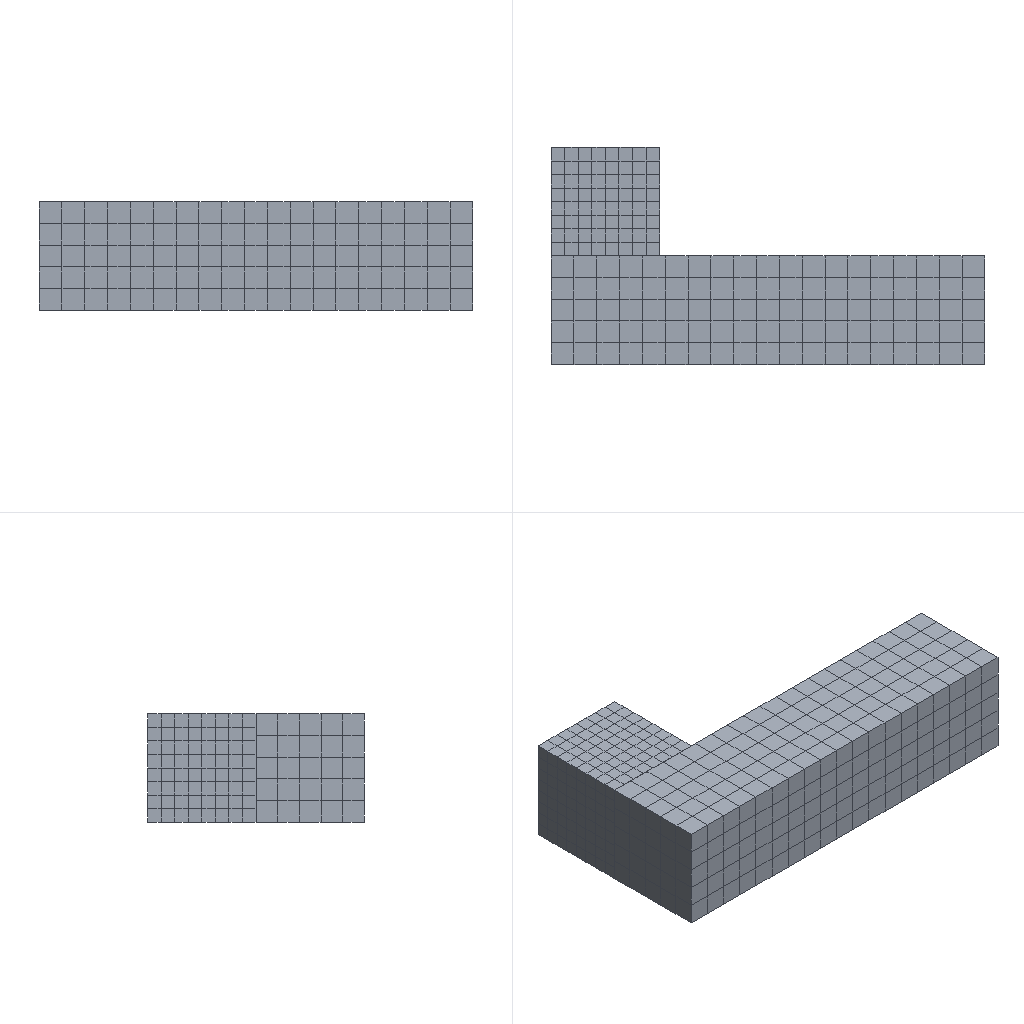Simulation study | ansys workbench
Set-up summary:
category,name,step,type,value,unit,region
solver,ansys_workbench
units,mm-N-s-tonne (MPa),,stated,"/units,MPA"
analysis,LS1,,transient
load_step,LS1,LS1,transient,nsubst=25; time=0.015
mesh,nodes,,,5277
mesh,elements,,,1369
element_type,SOLID186,,,987
element_type,TARGE170,,,159
element_type,CONTA174,,,159
element_type,SURF154,,,64
material,Structural Steel,,E,200000,tonne s^-2 mm^-1
material,Structural Steel,,nu,0.3
material,Structural Steel,,density,7.85e-09,tonne mm^-3
material,Structural Steel,,conductivity,60.5,tonne mm s^-3 C^-1
material,Structural Steel,,specific_heat,4.34e+08,mm^2 s^-2 C^-1
material,Structural Steel,,cte,1.2e-05,C^-1
material,Structural Steel,,permeability,10000
material,Structural Steel,,resistivity,0.00017,ohm mm
load,"Define Pressure Using Surface Effect Elements ""Pressure""",LS1,pressure,40,,SURF154 #5
load,Component For All Non-Zero UX Displacements,LS1,body load temp,22,,all
bc,Constant Zero Displacement X,model,fixed,[dofs=UX],,_DISPZEROUX
bc,Constant Zero Displacement Y,model,fixed,[dofs=UY],,_DISPZEROUY
bc,Constant Zero Displacement Z,model,fixed,[dofs=UZ],,_DISPZEROUZ
bc,Set Displacements,LS1,prescribed ux,15 [dofs=UX],,_CM48UX_XP
contact,Frictional - 1 To 2,,standard (frictionless/frictional),friction=0.2; element=CONTA174
named_set,_DISPZEROUX,,node,334
named_set,_DISPZEROUY,,node,334
named_set,_DISPZEROUZ,,node,559
named_set,_CM48UX_XP,,node,225
Ansys APDL input file, long lists of numbers shortened:
/batch
/config,noeldb,1     ! force off writing results to database
*get,_wallstrt,active,,time,wall
! ANSYS input file written by Workbench version 2023 R1
! File used for geometry attach:
/title,sk--Transient (B5)
! ****** Begin Custom Load Command Snippet ******
/COM, ACT Extensions:
/COM,     LSDYNA, 2023.1
/COM,/COM,     ANSYSMotion, 2023.1
/COM,
! ****** End   Custom Load Command Snippet ******
*DIM,_wb_ProjectScratch_dir,string,248
_wb_ProjectScratch_dir(1) = ''
*DIM,_wb_SolverFiles_dir,string,248
_wb_SolverFiles_dir(1) = ''
*DIM,_wb_userfiles_dir,string,248
_wb_userfiles_dir(1) = ''
/com,--- Data in consistent NMM units. See Solving Units in the help system for more information.
/units,MPA
/nopr
/wb,file,start              !  signify a WB generated input file
/prep7
! Turn off shape checking because checks already performed inside WB mesher.
! See help system for more information.
SHPP,OFF,,NOWARN
/nolist
etcon,set             ! allow ANSYS to choose best KEYOP's for 180x elements, resets any applicable keyopt to MAPDL defaults
/com,*********** Nodes for the whole assembly ***********
nblock,3,,5804
(1i9,3e20.9e3)
        1     4.375000000E+00     4.375000000E+00     4.375000000E+00
! (5276 more lines like these left out)
-1
/wb,elem,start            !  set before creation of elements
/com,*********** Elements for Body 1 "1" ***********
et,1,186
keyo,1,2,1          ! set full integration on SOLID186
eblock,19,solid,,512
(19i9)
        1        1        1        1        0        0        0        0       20        0        1        1      652      672      674      392      665      673      723
! (1023 more lines like these left out)
-1
/com,*********** Elements for Body 2 "2" ***********
et,2,186
keyo,2,2,1          ! set full integration on SOLID186
eblock,19,solid,,475
(19i9)
        2        2        2        2        0        0        0        0       20        0      513     2674     3321     3175     3157     3033     3393     3174     3170
! (949 more lines like these left out)
-1
/wb,elem,end               !  done creating elements
/com,*********** Send User Defined Coordinate System(s) ***********
csys,0
toffst,273.15,  ! Temperature offset from absolute zero
/com,*********** Set Reference Temperature ***********
tref,22.
/wb,mat,start              !  starting to send materials
/com,*********** Send Materials ***********
Temperature = 'TEMP' ! Temperature
MP,DENS,1,7.85e-09,	! tonne mm^-3
MP,ALPX,1,1.2e-05,	! C^-1
MP,C,1,434000000,	! mm^2 s^-2 C^-1
MP,KXX,1,60.5,	! tonne mm s^-3 C^-1
MP,RSVX,1,0.00017,	! ohm mm
MP,EX,1,200000,	! tonne s^-2 mm^-1
MP,NUXY,1,0.3,
MP,MURX,1,10000,
Temperature = 'TEMP' ! Temperature
MP,DENS,2,7.85e-09,	! tonne mm^-3
MP,ALPX,2,1.2e-05,	! C^-1
MP,C,2,434000000,	! mm^2 s^-2 C^-1
MP,KXX,2,60.5,	! tonne mm s^-3 C^-1
MP,RSVX,2,0.00017,	! ohm mm
MP,EX,2,200000,	! tonne s^-2 mm^-1
MP,NUXY,2,0.3,
MP,MURX,2,10000,
/wb,mat,end                !  done sending materials
! ****** Begin Command Snippet ******
*dim,matids,,1
*set,matids(1),1
*set,matid,1
*dim,typeids,,1
*set,typeids(1),1
!   Commands inserted into this file will be executed just after material definitions in /PREP7.
!   The material number for this body is equal to the parameter "matid" if it's not a part of a Material Assignment.
!   The element type numbers for this body can be referenced using the 1-D array parameter "typeids".
!   Active UNIT system in Workbench when this object was created:  Metric (mm, kg, N, s, mV, mA)
!   NOTE:  Any data that requires units (such as mass) is assumed to be in the consistent solver unit system.
!                See Solving Units in the help system for more information.
et,matid,solid226,11
*set, matids, ,
*set, typeids, ,
! ****** End   Command Snippet ******
! ****** Begin Command Snippet ******
*dim,matids,,1
*set,matids(1),2
*set,matid,2
*dim,typeids,,1
*set,typeids(1),2
!   Commands inserted into this file will be executed just after material definitions in /PREP7.
!   The material number for this body is equal to the parameter "matid" if it's not a part of a Material Assignment.
!   The element type numbers for this body can be referenced using the 1-D array parameter "typeids".
!   Active UNIT system in Workbench when this object was created:  Metric (mm, kg, N, s, mV, mA)
!   NOTE:  Any data that requires units (such as mass) is assumed to be in the consistent solver unit system.
!                See Solving Units in the help system for more information.
et,matid,solid226,11
*set, matids, ,
*set, typeids, ,
! ****** End   Command Snippet ******
!************************* Model Summary ********************
!1,	Structural Steel,	matid,	1
!2,	Structural Steel,	matid,	2
!************************* End Model Summary ********************
! get the diagonal of the bounding box. Needed later for other things
*get,_xmin,node,,mnloc,x
*get,_ymin,node,,mnloc,y
*get,_zmin,node,,mnloc,z
*get,_xmax,node,,mxloc,x
*get,_ymax,node,,mxloc,y
*get,_zmax,node,,mxloc,z
_ASMDIAG=(_xmax-_xmin)*(_xmax-_xmin)+(_ymax-_ymin)*(_ymax-_ymin)+(_zmax-_zmin)*(_zmax-_zmin)
_ASMDIAG=SQRT(_ASMDIAG)
/wb,contact,start          !  starting to send contact
/com,*********** Create Contact "Frictional - 1 To 2" ***********
/com,            Real Constant Set For Above Contact Is 4 & 3
*set,tid,4
*set,cid,3
r,tid
r,cid
et,tid,170
et,cid,174
eblock,10,,,64
(15i9)
     1802        4        4        4        0      602      546      458      457     2339     2164     2161     2162
! (63 more lines like these left out)
-1
eblock,10,,,64
(15i9)
     1866        3        3        3        0      602      546      458      457     2339     2164     2161     2162
! (63 more lines like these left out)
-1
eblock,10,,,95
(15i9)
     1930        3        4        3        0     3147     3184     3183     3148     4834     4904     4836     4833
! (94 more lines like these left out)
-1
eblock,10,,,95
(15i9)
     2025        4        3        4        0     3147     3184     3183     3148     4834     4904     4836     4833
! (94 more lines like these left out)
-1
keyo,cid,8,2               ! auto create asymmetric contact (from Program Controlled setting)
keyo,cid,10,0              ! adjust contact stiffness each NR iteration (from Program Controlled setting)
keyo,cid,12,0              ! standard contact
mp,mu,cid,0.2       ! unitless
keyo,cid,2,0               ! augmented Lagrange (from Program Controlled setting)
keyo,cid,4,0               ! on Gauss point (from Program Controlled setting)
keyo,cid,9,0               ! use real geometry with stepped effects
keyo,cid,7,0               ! No Prediction
rmod,tid,3,1.       ! FKN
rmod,tid,5,0.       ! ICONT
rmod,tid,6,0.       ! PINB
rmod,tid,10,0.      ! CNOF
rmod,tid,12,0.      ! FKT
rmod,tid,36,30      ! WB DSID
rmod,cid,3,1.       ! FKN
rmod,cid,5,0.       ! ICONT
rmod,cid,6,0.       ! PINB
rmod,cid,10,0.      ! CNOF
rmod,cid,12,0.      ! FKT
rmod,cid,36,30      ! WB DSID
! ****** Begin Command Snippet ******
!   Commands inserted into this file will be executed just after the contact region definition.
!   The type and mat number for the contact type is equal to the parameter "cid".
!   The type and mat number for the target type is equal to the parameter "tid".
!   The real number for an asymmetric contact pair is equal to the parameter "cid".
!   The real numbers for symmetric contact pairs are equal to the parameters "cid" and "tid".
!   Active UNIT system in Workbench when this object was created:  Metric (mm, kg, N, s, mV, mA)
!   NOTE:  Any data that requires units (such as mass) is assumed to be in the consistent solver unit system.
!                See Solving Units in the help system for more information.
keyopt,cid,1,1
! ****** End   Command Snippet ******
nsel,all
esel,all
/wb,contact,end            !  done creating contacts
/golist
/wb,load,start             !  starting to send loads
/com,******* Constant Zero Displacement X *******
CMBLOCK,_DISPZEROUX,NODE,      334
(8i10)
      3106      3107      3108      3109      3110      3111      3112      3113
! (41 more lines like these left out)
cmsel,s,_DISPZEROUX
d,all,ux,0
nsel,all
/com,******* Constant Zero Displacement Y *******
CMBLOCK,_DISPZEROUY,NODE,      334
(8i10)
      3106      3107      3108      3109      3110      3111      3112      3113
! (41 more lines like these left out)
cmsel,s,_DISPZEROUY
d,all,uy,0
nsel,all
/com,******* Constant Zero Displacement Z *******
CMBLOCK,_DISPZEROUZ,NODE,      559
(8i10)
       449       450       451       452       453       454       455       456
! (69 more lines like these left out)
cmsel,s,_DISPZEROUZ
d,all,uz,0
nsel,all
/com,*********** Define Pressure Using Surface Effect Elements "Pressure" ***********
et,5,154
mat,5
eblock,10,,,64
(15i9)
     2120        5        5        5        0      672      674      723      673     2575     2579     2576     2574
! (63 more lines like these left out)
-1
esel,s,type,,5
keyop,5,7,0                ! Use deformed area for application of load
esel,all
/com,*********** Create Displacement Tables and Functions ******
*DIM,_loadvari48xp,TABLE,2,1,1,TIME
! Time values
*TAXIS,_loadvari48xp(1),1,0.,1.5e-002
! Load values
_loadvari48xp(1,1,1) = 0.
_loadvari48xp(2,1,1) = 15.
*DIM,_loadvari48xn,TABLE,2,1,1,TIME
! Time values
*TAXIS,_loadvari48xn(1),1,0.,1.5e-002
! Load values
_loadvari48xn(1,1,1) = 0.
_loadvari48xn(2,1,1) = -15.
esel,all
/gst,on,on
fini
*get,_numnode,node,0,count
*get,_numelem,elem,0,count
*get, _MAXELEMNUM, elem, 0, NUM, MAX
*get, _MAXNODENUM, node, 0, NUM, MAX
*get, _MAXELEMTYPE, etyp, 0, NUM, MAX
*get, _MAXREALCONST, rcon, 0, NUM, MAX
/go
/wb,load,end               !  done creating loads
/com,--- Number of total nodes = %_numnode%
/com,--- Number of contact elements = 382
/com,--- Number of spring elements = 0
/com,--- Number of bearing elements = 0
/com,--- Number of solid elements = 987
/com,--- Number of condensed parts = 0
/com,--- Number of total elements = %_numelem%
*get,_wallbsol,active,,time,wall
/com,****************************************************************************
/com,*************************    SOLUTION       ********************************
/com,****************************************************************************
/solu
antype,4                   ! transient analysis
nlgeom,on                  ! Turn on Large Deformation Effects
kbc,1                      ! stepped BC's
_thickRatio=  1     ! Ratio of thick parts in the model
eqsl,pcg,1e-8,,,,,,1
cntr,print,1               ! print out contact info and also make no initial contact an error
dmpoption,emat,no             ! Don't combine emat file for DANSYS
dmpoption,esav,no             ! Don't combine esav file for DANSYS
trnopt,full,,,,,hht        ! HHT time integration method
tintp, mosp			! Choose transient integration settings for moderate speed application
nldiag,cont,iter           ! print out contact info each equilibrium iteration
rescontrol,define,last,last,,dele	   ! Program Controlled
/com,****************************************************
/com,******************* SOLVE FOR LS 1 OF 1 ****************
esel,s,type,,5
nsle
sf,all,pres,40.
nsel,all
esel,all
/com,*** Set Displacements ***
CMBLOCK,_CM48UX_XP,NODE,      225
(8i10)
       449       450       451       452       453       454       455       456
! (28 more lines like these left out)
cmsel,s,_CM48UX_XP
d,all,ux,%_loadvari48xp%
nsel,all
/com,*** Component For All Non-Zero UX Displacements ***
cmsel,s,_CM48ux_xp
cm,_DISPNONZEROUX,NODE
nsel,all
esel,all
/nopr
/gopr
autots,off                 ! User turned off automatic time stepping
nsub,25,25,25
time,1.5e-002
timint,on                  ! Turn on time integration effects
outres,erase
outres,all,none
outres,nsol,all,
outres,rsol,all
outres,eangl,all
outres,etmp,all
outres,veng,all
outres,strs,all,
outres,epel,all,
outres,eppl,all,
outres,cont,all,
outres,v,all,
outres,a,all,
cnvtol,,-1,29               ! User deleted Convergence, engy
! ****** Begin Command Snippet ******
!   Commands inserted into this file will be executed just prior to the ANSYS SOLVE command.
!   These commands may supersede command settings set by Workbench.
!   Active UNIT system in Workbench when this object was created:  Metric (mm, kg, N, s, mV, mA)
!   NOTE:  Any data that requires units (such as mass) is assumed to be in the consistent solver unit system.
!                See Solving Units in the help system for more information.
/SOLU
ALLSEL
TUNIF,22
TREF,22
! ****** End   Command Snippet ******
! *********** WB SOLVE COMMAND ***********
! check interactive state
*get,ANSINTER_,active,,int
*if,ANSINTER_,ne,0,then
/eof
*endif
solve
/com *************** Write FE CONNECTORS *********
CEWRITE,file,ce,,INTE
/com,****************************************************
/com,*************** FINISHED SOLVE FOR LS 1 *************
*get,_wallasol,active,,time,wall
/nopr
*get,_numnode,node,0,count
*get,_numelem,elem,0,count
*get, _MAXELEMNUM, elem, 0, NUM, MAX
*get, _MAXNODENUM, node, 0, NUM, MAX,,,INTERNAL
*get, _MAXELEMTYPE, etyp, 0, NUM, MAX
*get, _MAXREALCONST, rcon, 0, NUM, MAX
*get,_NSOLTHREADS,active,0,ntfs
*get,_NSOLPROCESSES,active,0,npfs
/gopr
*get,_PCGITER,active,,solu,cgiter
/post1
xmlo,ENCODING,ISO-8859-1
xmlo,parm
/xml,parm,xml
fini
/gopr
*get,_walldone,active,,time,wall
_preptime=(_wallbsol-_wallstrt)*3600
_solvtime=(_wallasol-_wallbsol)*3600
_posttime=(_walldone-_wallasol)*3600
_totaltim=(_walldone-_wallstrt)*3600
*get,_dlbratio,active,0,solu,dlbr
*get,_combtime,active,0,solu,comb
*get,_ssmode,active,0,solu,ssmm
*get,_ndofs,active,0,solu,ndof
*get,_sol_end_time,active,0,set,time
*if,_sol_end_time,eq,0.015,then
/fclean				!clean distributed files
*endif
/com,--- Total number of nodes = %_numnode%
/com,--- Total number of elements = %_numelem%
/com,--- Element load balance ratio = %_dlbratio%
/com,--- Time to combine distributed files = %_combtime%
/com,--- Sparse memory mode = %_ssmode%
/com,--- Number of DOF = %_ndofs%
/wb,file,end               ! done with WB generated input
Results summary:
result,analyses[0].index,,,1
result,analyses[0].system,,,SYS
result,analyses[0].deck,,,deck.dat
result,analyses[0].solve_status,,,completed
result,analyses[0].analysis_type,,,static
result,analyses[0].physics,,,mechanical
result,analyses[0].unit_system,,,"NMM: mm, ton, N, s, mV, mA, degC"
result,analyses[0].n_sets,,,25
result,analyses[0].load_steps[0].set,set=25,,25
result,analyses[0].load_steps[0].time_or_freq,set=25,,0.015
result,analyses[0].load_steps[0].max_displacement_magnitude,set=25,,15
result,analyses[0].load_steps[0].max_von_mises_nodal,set=25,,224.697
result,analyses[0].load_steps[0].reaction_force_sum_xyz[1],set=25,,1.522
result,analyses[0].load_steps[0].reaction_force_sum_xyz[2],set=25,,1000.05
result,analyses[0].load_steps[0].reaction_force_sum_xyz[3],set=25,,-8.50577e-11
result,analyses[0].load_steps[0].max_temperature,set=25,,81.872
result,analyses[0].load_steps[0].min_temperature,set=25,,20.964
result,geometry_export[0][0],,,.step
result,geometry_export[0][1],,,ok
result,geometry_export[0][2],,,2